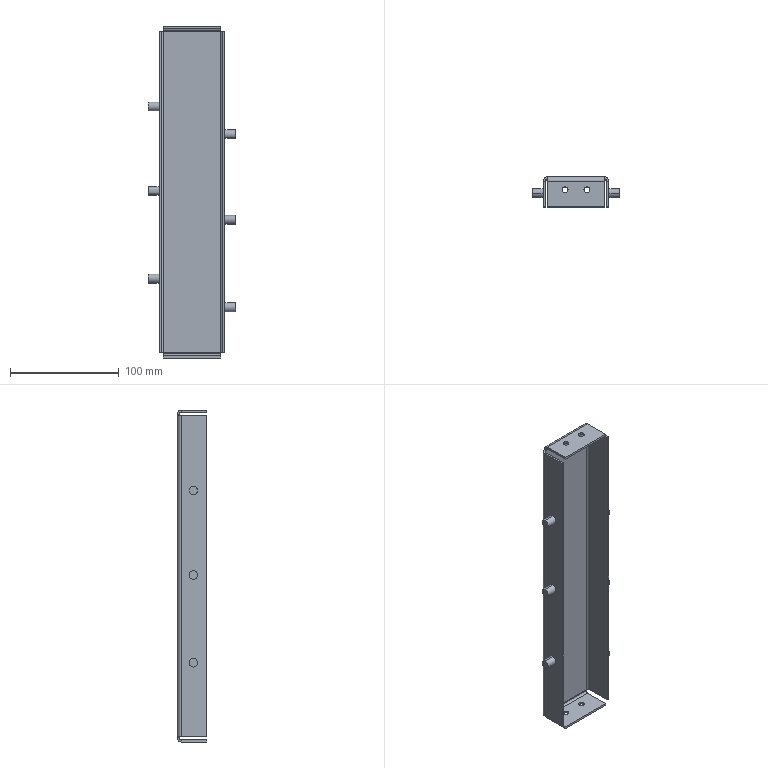Part | STEP file | 64605046 | 1 solid | 72 faces | box 80.6 x 27.5 x 306 mm | volume 73522 mm3 | plane 44 | cylinder 28 | commonest cylinder face diameters 8 x16 5.4 x8 4 x4